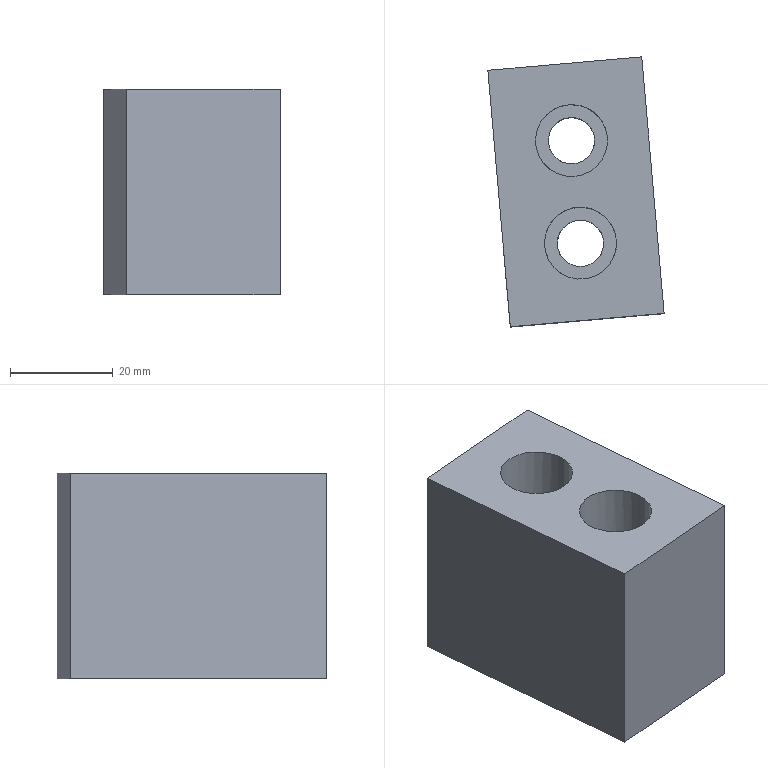Part | NX | features solid 2 | 1 solid | 12 faces | box 34.244 x 52.424 x 40 mm | volume 51298 mm3 | plane 8 | cylinder 4 | commonest cylinder face diameters 9 x2 14 x2
STEP:
#1=CARTESIAN_POINT('',(763.588,512.986,-265.));
#2=VERTEX_POINT('',#1);
#3=CARTESIAN_POINT('',(763.588,508.486,-265.));
#4=DIRECTION('',(0.,0.,1.));
#5=DIRECTION('',(0.,1.,0.));
#6=AXIS2_PLACEMENT_3D('',#3,#4,#5);
#7=CIRCLE('',#6,4.5);
#8=EDGE_CURVE('',#2,#2,#7,.F.);
#9=ORIENTED_EDGE('',*,*,#8,.F.);
#10=EDGE_LOOP('',(#9));
#11=FACE_BOUND('',#10,.T.);
#12=CARTESIAN_POINT('',(747.338,522.122,-265.));
#13=VERTEX_POINT('',#12);
#14=CARTESIAN_POINT('',(751.696,472.312,-265.));
#15=VERTEX_POINT('',#14);
#16=CARTESIAN_POINT('',(747.338,522.122,-265.));
#17=DIRECTION('',(-0.08716,0.9962,0.));
#18=VECTOR('',#17,1000.);
#19=LINE('',#16,#18);
#20=EDGE_CURVE('',#13,#15,#19,.F.);
#21=ORIENTED_EDGE('',*,*,#20,.F.);
#22=CARTESIAN_POINT('',(777.224,524.736,-265.));
#23=VERTEX_POINT('',#22);
#24=CARTESIAN_POINT('',(744.847,521.904,-265.));
#25=DIRECTION('',(0.9962,0.08716,0.));
#26=VECTOR('',#25,1000.);
#27=LINE('',#24,#26);
#28=EDGE_CURVE('',#23,#13,#27,.F.);
#29=ORIENTED_EDGE('',*,*,#28,.F.);
#30=CARTESIAN_POINT('',(781.582,474.927,-265.));
#31=VERTEX_POINT('',#30);
#32=CARTESIAN_POINT('',(777.224,524.736,-265.));
#33=DIRECTION('',(-0.08716,0.9962,0.));
#34=VECTOR('',#33,1000.);
#35=LINE('',#32,#34);
#36=EDGE_CURVE('',#23,#31,#35,.F.);
#37=ORIENTED_EDGE('',*,*,#36,.T.);
#38=CARTESIAN_POINT('',(749.205,472.094,-265.));
#39=DIRECTION('',(-0.9962,-0.08716,0.));
#40=VECTOR('',#39,1000.);
#41=LINE('',#38,#40);
#42=EDGE_CURVE('',#31,#15,#41,.T.);
#43=ORIENTED_EDGE('',*,*,#42,.T.);
#44=EDGE_LOOP('',(#21,#29,#37,#43));
#45=FACE_BOUND('',#44,.T.);
#46=CARTESIAN_POINT('',(765.331,493.062,-265.));
#47=VERTEX_POINT('',#46);
#48=CARTESIAN_POINT('',(765.331,488.562,-265.));
#49=DIRECTION('',(0.,0.,1.));
#50=DIRECTION('',(0.,1.,0.));
#51=AXIS2_PLACEMENT_3D('',#48,#49,#50);
#52=CIRCLE('',#51,4.5);
#53=EDGE_CURVE('',#47,#47,#52,.F.);
#54=ORIENTED_EDGE('',*,*,#53,.F.);
#55=EDGE_LOOP('',(#54));
#56=FACE_BOUND('',#55,.T.);
#57=CARTESIAN_POINT('',(744.847,521.904,-265.));
#58=DIRECTION('',(0.,0.,-1.));
#59=DIRECTION('',(0.08716,-0.9962,0.));
#60=AXIS2_PLACEMENT_3D('',#57,#58,#59);
#61=PLANE('',#60);
#62=ADVANCED_FACE('',(#11,#45,#56),#61,.T.);
#63=CARTESIAN_POINT('',(763.588,515.486,-225.));
#64=VERTEX_POINT('',#63);
#65=CARTESIAN_POINT('',(763.588,508.486,-225.));
#66=DIRECTION('',(0.,0.,1.));
#67=DIRECTION('',(0.,1.,0.));
#68=AXIS2_PLACEMENT_3D('',#65,#66,#67);
#69=CIRCLE('',#68,7.);
#70=EDGE_CURVE('',#64,#64,#69,.T.);
#71=ORIENTED_EDGE('',*,*,#70,.F.);
#72=EDGE_LOOP('',(#71));
#73=FACE_BOUND('',#72,.T.);
#74=CARTESIAN_POINT('',(777.224,524.736,-225.));
#75=VERTEX_POINT('',#74);
#76=CARTESIAN_POINT('',(781.582,474.927,-225.));
#77=VERTEX_POINT('',#76);
#78=CARTESIAN_POINT('',(777.224,524.736,-225.));
#79=DIRECTION('',(0.08716,-0.9962,0.));
#80=VECTOR('',#79,1000.);
#81=LINE('',#78,#80);
#82=EDGE_CURVE('',#75,#77,#81,.T.);
#83=ORIENTED_EDGE('',*,*,#82,.F.);
#84=CARTESIAN_POINT('',(747.338,522.122,-225.));
#85=VERTEX_POINT('',#84);
#86=CARTESIAN_POINT('',(744.847,521.904,-225.));
#87=DIRECTION('',(0.9962,0.08716,0.));
#88=VECTOR('',#87,1000.);
#89=LINE('',#86,#88);
#90=EDGE_CURVE('',#75,#85,#89,.F.);
#91=ORIENTED_EDGE('',*,*,#90,.T.);
#92=CARTESIAN_POINT('',(751.696,472.312,-225.));
#93=VERTEX_POINT('',#92);
#94=CARTESIAN_POINT('',(747.338,522.122,-225.));
#95=DIRECTION('',(0.08716,-0.9962,0.));
#96=VECTOR('',#95,1000.);
#97=LINE('',#94,#96);
#98=EDGE_CURVE('',#85,#93,#97,.T.);
#99=ORIENTED_EDGE('',*,*,#98,.T.);
#100=CARTESIAN_POINT('',(749.205,472.094,-225.));
#101=DIRECTION('',(0.9962,0.08716,0.));
#102=VECTOR('',#101,1000.);
#103=LINE('',#100,#102);
#104=EDGE_CURVE('',#77,#93,#103,.F.);
#105=ORIENTED_EDGE('',*,*,#104,.F.);
#106=EDGE_LOOP('',(#83,#91,#99,#105));
#107=FACE_BOUND('',#106,.T.);
#108=CARTESIAN_POINT('',(765.331,495.562,-225.));
#109=VERTEX_POINT('',#108);
#110=CARTESIAN_POINT('',(765.331,488.562,-225.));
#111=DIRECTION('',(0.,0.,1.));
#112=DIRECTION('',(0.,1.,0.));
#113=AXIS2_PLACEMENT_3D('',#110,#111,#112);
#114=CIRCLE('',#113,7.);
#115=EDGE_CURVE('',#109,#109,#114,.T.);
#116=ORIENTED_EDGE('',*,*,#115,.F.);
#117=EDGE_LOOP('',(#116));
#118=FACE_BOUND('',#117,.T.);
#119=CARTESIAN_POINT('',(744.847,521.904,-225.));
#120=DIRECTION('',(0.,0.,-1.));
#121=DIRECTION('',(0.08716,-0.9962,0.));
#122=AXIS2_PLACEMENT_3D('',#119,#120,#121);
#123=PLANE('',#122);
#124=ADVANCED_FACE('',(#73,#107,#118),#123,.F.);
#125=ORIENTED_EDGE('',*,*,#98,.F.);
#126=CARTESIAN_POINT('',(747.338,522.122,-275.));
#127=DIRECTION('',(0.,0.,1.));
#128=VECTOR('',#127,1000.);
#129=LINE('',#126,#128);
#130=EDGE_CURVE('',#13,#85,#129,.T.);
#131=ORIENTED_EDGE('',*,*,#130,.F.);
#132=ORIENTED_EDGE('',*,*,#20,.T.);
#133=CARTESIAN_POINT('',(751.696,472.312,-275.));
#134=DIRECTION('',(0.,0.,-1.));
#135=VECTOR('',#134,1000.);
#136=LINE('',#133,#135);
#137=EDGE_CURVE('',#15,#93,#136,.F.);
#138=ORIENTED_EDGE('',*,*,#137,.T.);
#139=EDGE_LOOP('',(#125,#131,#132,#138));
#140=FACE_BOUND('',#139,.T.);
#141=CARTESIAN_POINT('',(747.338,522.122,-275.));
#142=DIRECTION('',(0.9962,0.08716,0.));
#143=DIRECTION('',(0.08716,-0.9962,0.));
#144=AXIS2_PLACEMENT_3D('',#141,#142,#143);
#145=PLANE('',#144);
#146=ADVANCED_FACE('',(#140),#145,.F.);
#147=ORIENTED_EDGE('',*,*,#36,.F.);
#148=CARTESIAN_POINT('',(777.224,524.736,-275.));
#149=DIRECTION('',(0.,0.,1.));
#150=VECTOR('',#149,1000.);
#151=LINE('',#148,#150);
#152=EDGE_CURVE('',#23,#75,#151,.T.);
#153=ORIENTED_EDGE('',*,*,#152,.T.);
#154=ORIENTED_EDGE('',*,*,#82,.T.);
#155=CARTESIAN_POINT('',(781.582,474.927,-275.));
#156=DIRECTION('',(0.,0.,-1.));
#157=VECTOR('',#156,1000.);
#158=LINE('',#155,#157);
#159=EDGE_CURVE('',#31,#77,#158,.F.);
#160=ORIENTED_EDGE('',*,*,#159,.F.);
#161=EDGE_LOOP('',(#147,#153,#154,#160));
#162=FACE_BOUND('',#161,.T.);
#163=CARTESIAN_POINT('',(777.224,524.736,-275.));
#164=DIRECTION('',(0.9962,0.08716,0.));
#165=DIRECTION('',(0.08716,-0.9962,0.));
#166=AXIS2_PLACEMENT_3D('',#163,#164,#165);
#167=PLANE('',#166);
#168=ADVANCED_FACE('',(#162),#167,.T.);
#169=ORIENTED_EDGE('',*,*,#152,.F.);
#170=ORIENTED_EDGE('',*,*,#28,.T.);
#171=ORIENTED_EDGE('',*,*,#130,.T.);
#172=ORIENTED_EDGE('',*,*,#90,.F.);
#173=EDGE_LOOP('',(#169,#170,#171,#172));
#174=FACE_BOUND('',#173,.T.);
#175=CARTESIAN_POINT('',(744.847,521.904,-275.));
#176=DIRECTION('',(0.08716,-0.9962,0.));
#177=DIRECTION('',(0.,0.,1.));
#178=AXIS2_PLACEMENT_3D('',#175,#176,#177);
#179=PLANE('',#178);
#180=ADVANCED_FACE('',(#174),#179,.F.);
#181=CARTESIAN_POINT('',(768.02,509.267,-245.));
#182=VERTEX_POINT('',#181);
#183=CARTESIAN_POINT('',(763.588,508.486,-245.));
#184=DIRECTION('',(0.,0.,-1.));
#185=DIRECTION('',(0.9848,0.1736,0.));
#186=AXIS2_PLACEMENT_3D('',#183,#184,#185);
#187=CIRCLE('',#186,4.5);
#188=EDGE_CURVE('',#182,#182,#187,.T.);
#189=ORIENTED_EDGE('',*,*,#188,.F.);
#190=EDGE_LOOP('',(#189));
#191=FACE_BOUND('',#190,.T.);
#192=ORIENTED_EDGE('',*,*,#8,.T.);
#193=EDGE_LOOP('',(#192));
#194=FACE_BOUND('',#193,.T.);
#195=CARTESIAN_POINT('',(763.588,508.486,-245.));
#196=DIRECTION('',(0.,0.,-1.));
#197=DIRECTION('',(0.9848,0.1736,0.));
#198=AXIS2_PLACEMENT_3D('',#195,#196,#197);
#199=CYLINDRICAL_SURFACE('',#198,4.5);
#200=ADVANCED_FACE('',(#191,#194),#199,.F.);
#201=CARTESIAN_POINT('',(756.695,507.271,-245.));
#202=VERTEX_POINT('',#201);
#203=CARTESIAN_POINT('',(763.588,508.486,-245.));
#204=DIRECTION('',(0.,0.,1.));
#205=DIRECTION('',(-0.9848,-0.1736,0.));
#206=AXIS2_PLACEMENT_3D('',#203,#204,#205);
#207=CIRCLE('',#206,7.);
#208=EDGE_CURVE('',#202,#202,#207,.T.);
#209=ORIENTED_EDGE('',*,*,#208,.F.);
#210=EDGE_LOOP('',(#209));
#211=FACE_BOUND('',#210,.T.);
#212=ORIENTED_EDGE('',*,*,#70,.T.);
#213=EDGE_LOOP('',(#212));
#214=FACE_BOUND('',#213,.T.);
#215=CARTESIAN_POINT('',(763.588,508.486,-245.));
#216=DIRECTION('',(0.,0.,1.));
#217=DIRECTION('',(-0.9848,-0.1736,0.));
#218=AXIS2_PLACEMENT_3D('',#215,#216,#217);
#219=CYLINDRICAL_SURFACE('',#218,7.);
#220=ADVANCED_FACE('',(#211,#214),#219,.F.);
#221=ORIENTED_EDGE('',*,*,#188,.T.);
#222=EDGE_LOOP('',(#221));
#223=FACE_BOUND('',#222,.T.);
#224=ORIENTED_EDGE('',*,*,#208,.T.);
#225=EDGE_LOOP('',(#224));
#226=FACE_BOUND('',#225,.T.);
#227=CARTESIAN_POINT('',(763.588,508.486,-245.));
#228=DIRECTION('',(0.,0.,-1.));
#229=DIRECTION('',(0.9848,0.1736,0.));
#230=AXIS2_PLACEMENT_3D('',#227,#228,#229);
#231=PLANE('',#230);
#232=ADVANCED_FACE('',(#223,#226),#231,.F.);
#233=CARTESIAN_POINT('',(769.831,488.562,-245.));
#234=VERTEX_POINT('',#233);
#235=CARTESIAN_POINT('',(765.331,488.562,-245.));
#236=DIRECTION('',(0.,0.,1.));
#237=DIRECTION('',(1.,0.,0.));
#238=AXIS2_PLACEMENT_3D('',#235,#236,#237);
#239=CIRCLE('',#238,4.5);
#240=EDGE_CURVE('',#234,#234,#239,.T.);
#241=ORIENTED_EDGE('',*,*,#240,.F.);
#242=EDGE_LOOP('',(#241));
#243=FACE_BOUND('',#242,.T.);
#244=CARTESIAN_POINT('',(758.331,488.562,-245.));
#245=VERTEX_POINT('',#244);
#246=CARTESIAN_POINT('',(765.331,488.562,-245.));
#247=DIRECTION('',(0.,0.,-1.));
#248=DIRECTION('',(-1.,0.,0.));
#249=AXIS2_PLACEMENT_3D('',#246,#247,#248);
#250=CIRCLE('',#249,7.);
#251=EDGE_CURVE('',#245,#245,#250,.T.);
#252=ORIENTED_EDGE('',*,*,#251,.F.);
#253=EDGE_LOOP('',(#252));
#254=FACE_BOUND('',#253,.T.);
#255=CARTESIAN_POINT('',(765.331,488.562,-245.));
#256=DIRECTION('',(0.,0.,-1.));
#257=DIRECTION('',(1.,0.,0.));
#258=AXIS2_PLACEMENT_3D('',#255,#256,#257);
#259=PLANE('',#258);
#260=ADVANCED_FACE('',(#243,#254),#259,.F.);
#261=ORIENTED_EDGE('',*,*,#240,.T.);
#262=EDGE_LOOP('',(#261));
#263=FACE_BOUND('',#262,.T.);
#264=ORIENTED_EDGE('',*,*,#53,.T.);
#265=EDGE_LOOP('',(#264));
#266=FACE_BOUND('',#265,.T.);
#267=CARTESIAN_POINT('',(765.331,488.562,-245.));
#268=DIRECTION('',(0.,0.,-1.));
#269=DIRECTION('',(1.,0.,0.));
#270=AXIS2_PLACEMENT_3D('',#267,#268,#269);
#271=CYLINDRICAL_SURFACE('',#270,4.5);
#272=ADVANCED_FACE('',(#263,#266),#271,.F.);
#273=ORIENTED_EDGE('',*,*,#251,.T.);
#274=EDGE_LOOP('',(#273));
#275=FACE_BOUND('',#274,.T.);
#276=ORIENTED_EDGE('',*,*,#115,.T.);
#277=EDGE_LOOP('',(#276));
#278=FACE_BOUND('',#277,.T.);
#279=CARTESIAN_POINT('',(765.331,488.562,-245.));
#280=DIRECTION('',(0.,0.,1.));
#281=DIRECTION('',(-1.,0.,0.));
#282=AXIS2_PLACEMENT_3D('',#279,#280,#281);
#283=CYLINDRICAL_SURFACE('',#282,7.);
#284=ADVANCED_FACE('',(#275,#278),#283,.F.);
#285=ORIENTED_EDGE('',*,*,#42,.F.);
#286=ORIENTED_EDGE('',*,*,#159,.T.);
#287=ORIENTED_EDGE('',*,*,#104,.T.);
#288=ORIENTED_EDGE('',*,*,#137,.F.);
#289=EDGE_LOOP('',(#285,#286,#287,#288));
#290=FACE_BOUND('',#289,.T.);
#291=CARTESIAN_POINT('',(749.205,472.094,-275.));
#292=DIRECTION('',(0.08716,-0.9962,0.));
#293=DIRECTION('',(0.,0.,1.));
#294=AXIS2_PLACEMENT_3D('',#291,#292,#293);
#295=PLANE('',#294);
#296=ADVANCED_FACE('',(#290),#295,.T.);
#297=CLOSED_SHELL('',(#62,#124,#146,#168,#180,#200,#220,#232,#260,#272,#284,#296));
#298=MANIFOLD_SOLID_BREP('',#297);
#299=(LENGTH_UNIT()NAMED_UNIT(*)SI_UNIT(.MILLI.,.METRE.));
#300=UNCERTAINTY_MEASURE_WITH_UNIT(LENGTH_MEASURE(0.00001),#299,'','');
#301=(NAMED_UNIT(*)PLANE_ANGLE_UNIT()SI_UNIT($,.RADIAN.));
#302=(NAMED_UNIT(*)SI_UNIT($,.STERADIAN.)SOLID_ANGLE_UNIT());
#303=(GEOMETRIC_REPRESENTATION_CONTEXT(3)GLOBAL_UNCERTAINTY_ASSIGNED_CONTEXT((#300))GLOBAL_UNIT_ASSIGNED_CONTEXT((#299,#301,#302))REPRESENTATION_CONTEXT('',''));
#304=ADVANCED_BREP_SHAPE_REPRESENTATION('',(#298),#303);